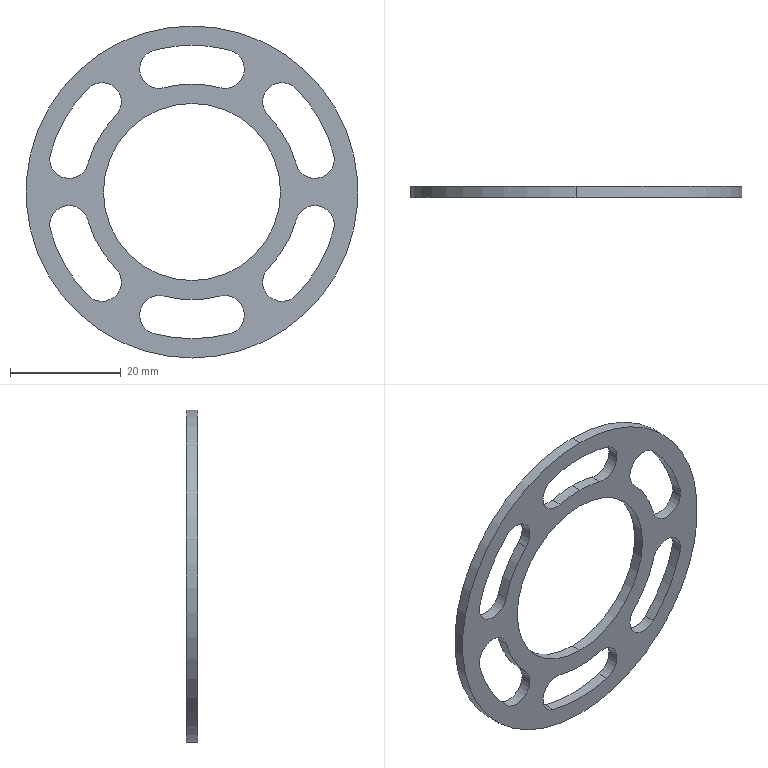Part | SolidWorks | features Extrusion 1, ICE 1 | 1 solid | 38 faces | box 60 x 2 x 60 mm | volume 2573 mm3 | cylinder 36 | plane 2 | commonest cylinder face diameters 7 x18 39 x7 53 x7 32 x2 60 x2
STEP:
#1=CARTESIAN_POINT('',(22.216,0.,-2.453));
#2=VERTEX_POINT('',#1);
#3=CARTESIAN_POINT('',(25.597,0.,-6.859));
#4=VERTEX_POINT('',#3);
#5=CARTESIAN_POINT('',(22.216,0.,-5.953));
#6=DIRECTION('',(0.,1.,0.));
#7=DIRECTION('',(0.,0.,1.));
#8=AXIS2_PLACEMENT_3D('',#5,#6,#7);
#9=CIRCLE('',#8,3.5);
#10=EDGE_CURVE('',#2,#4,#9,.T.);
#11=ORIENTED_EDGE('',*,*,#10,.F.);
#12=CARTESIAN_POINT('',(22.216,2.,-2.453));
#13=VERTEX_POINT('',#12);
#14=CARTESIAN_POINT('',(22.216,0.,-2.453));
#15=DIRECTION('',(0.,1.,0.));
#16=VECTOR('',#15,1000.);
#17=LINE('',#14,#16);
#18=EDGE_CURVE('',#2,#13,#17,.T.);
#19=ORIENTED_EDGE('',*,*,#18,.T.);
#20=CARTESIAN_POINT('',(25.597,2.,-6.859));
#21=VERTEX_POINT('',#20);
#22=CARTESIAN_POINT('',(22.216,2.,-5.953));
#23=DIRECTION('',(0.,1.,0.));
#24=DIRECTION('',(0.,0.,1.));
#25=AXIS2_PLACEMENT_3D('',#22,#23,#24);
#26=CIRCLE('',#25,3.5);
#27=EDGE_CURVE('',#13,#21,#26,.T.);
#28=ORIENTED_EDGE('',*,*,#27,.T.);
#29=CARTESIAN_POINT('',(25.597,0.,-6.859));
#30=DIRECTION('',(0.,1.,0.));
#31=VECTOR('',#30,1000.);
#32=LINE('',#29,#31);
#33=EDGE_CURVE('',#4,#21,#32,.T.);
#34=ORIENTED_EDGE('',*,*,#33,.F.);
#35=EDGE_LOOP('',(#11,#19,#28,#34));
#36=FACE_OUTER_BOUND('',#35,.T.);
#37=CARTESIAN_POINT('',(22.216,0.,-5.953));
#38=DIRECTION('',(0.,1.,0.));
#39=DIRECTION('',(0.,0.,1.));
#40=AXIS2_PLACEMENT_3D('',#37,#38,#39);
#41=CYLINDRICAL_SURFACE('',#40,3.5);
#42=ADVANCED_FACE('',(#36),#41,.F.);
#43=CARTESIAN_POINT('',(16.263,0.,19.763));
#44=VERTEX_POINT('',#43);
#45=CARTESIAN_POINT('',(18.738,0.,18.738));
#46=VERTEX_POINT('',#45);
#47=CARTESIAN_POINT('',(16.263,0.,16.263));
#48=DIRECTION('',(0.,1.,0.));
#49=DIRECTION('',(0.,0.,1.));
#50=AXIS2_PLACEMENT_3D('',#47,#48,#49);
#51=CIRCLE('',#50,3.5);
#52=EDGE_CURVE('',#44,#46,#51,.T.);
#53=ORIENTED_EDGE('',*,*,#52,.F.);
#54=CARTESIAN_POINT('',(16.263,2.,19.763));
#55=VERTEX_POINT('',#54);
#56=CARTESIAN_POINT('',(16.263,0.,19.763));
#57=DIRECTION('',(0.,1.,0.));
#58=VECTOR('',#57,1000.);
#59=LINE('',#56,#58);
#60=EDGE_CURVE('',#44,#55,#59,.T.);
#61=ORIENTED_EDGE('',*,*,#60,.T.);
#62=CARTESIAN_POINT('',(18.738,2.,18.738));
#63=VERTEX_POINT('',#62);
#64=CARTESIAN_POINT('',(16.263,2.,16.263));
#65=DIRECTION('',(0.,1.,0.));
#66=DIRECTION('',(0.,0.,1.));
#67=AXIS2_PLACEMENT_3D('',#64,#65,#66);
#68=CIRCLE('',#67,3.5);
#69=EDGE_CURVE('',#55,#63,#68,.T.);
#70=ORIENTED_EDGE('',*,*,#69,.T.);
#71=CARTESIAN_POINT('',(18.738,0.,18.738));
#72=DIRECTION('',(0.,1.,0.));
#73=VECTOR('',#72,1000.);
#74=LINE('',#71,#73);
#75=EDGE_CURVE('',#46,#63,#74,.T.);
#76=ORIENTED_EDGE('',*,*,#75,.F.);
#77=EDGE_LOOP('',(#53,#61,#70,#76));
#78=FACE_OUTER_BOUND('',#77,.T.);
#79=CARTESIAN_POINT('',(16.263,0.,16.263));
#80=DIRECTION('',(0.,1.,0.));
#81=DIRECTION('',(0.,0.,1.));
#82=AXIS2_PLACEMENT_3D('',#79,#80,#81);
#83=CYLINDRICAL_SURFACE('',#82,3.5);
#84=ADVANCED_FACE('',(#78),#83,.F.);
#85=CARTESIAN_POINT('',(0.,0.,26.5));
#86=VERTEX_POINT('',#85);
#87=CARTESIAN_POINT('',(6.859,0.,25.597));
#88=VERTEX_POINT('',#87);
#89=CARTESIAN_POINT('',(0.,0.,0.));
#90=DIRECTION('',(0.,1.,0.));
#91=DIRECTION('',(0.,0.,1.));
#92=AXIS2_PLACEMENT_3D('',#89,#90,#91);
#93=CIRCLE('',#92,26.5);
#94=EDGE_CURVE('',#86,#88,#93,.T.);
#95=ORIENTED_EDGE('',*,*,#94,.F.);
#96=CARTESIAN_POINT('',(0.,2.,26.5));
#97=VERTEX_POINT('',#96);
#98=CARTESIAN_POINT('',(0.,0.,26.5));
#99=DIRECTION('',(0.,1.,0.));
#100=VECTOR('',#99,1000.);
#101=LINE('',#98,#100);
#102=EDGE_CURVE('',#86,#97,#101,.T.);
#103=ORIENTED_EDGE('',*,*,#102,.T.);
#104=CARTESIAN_POINT('',(6.859,2.,25.597));
#105=VERTEX_POINT('',#104);
#106=CARTESIAN_POINT('',(0.,2.,0.));
#107=DIRECTION('',(0.,1.,0.));
#108=DIRECTION('',(0.,0.,1.));
#109=AXIS2_PLACEMENT_3D('',#106,#107,#108);
#110=CIRCLE('',#109,26.5);
#111=EDGE_CURVE('',#97,#105,#110,.T.);
#112=ORIENTED_EDGE('',*,*,#111,.T.);
#113=CARTESIAN_POINT('',(6.859,0.,25.597));
#114=DIRECTION('',(0.,1.,0.));
#115=VECTOR('',#114,1000.);
#116=LINE('',#113,#115);
#117=EDGE_CURVE('',#88,#105,#116,.T.);
#118=ORIENTED_EDGE('',*,*,#117,.F.);
#119=EDGE_LOOP('',(#95,#103,#112,#118));
#120=FACE_OUTER_BOUND('',#119,.T.);
#121=CARTESIAN_POINT('',(0.,0.,0.));
#122=DIRECTION('',(0.,1.,0.));
#123=DIRECTION('',(0.,0.,1.));
#124=AXIS2_PLACEMENT_3D('',#121,#122,#123);
#125=CYLINDRICAL_SURFACE('',#124,26.5);
#126=ADVANCED_FACE('',(#120),#125,.F.);
#127=CARTESIAN_POINT('',(0.,0.,19.5));
#128=VERTEX_POINT('',#127);
#129=CARTESIAN_POINT('',(-5.047,0.,18.836));
#130=VERTEX_POINT('',#129);
#131=CARTESIAN_POINT('',(0.,0.,0.));
#132=DIRECTION('',(0.,-1.,0.));
#133=DIRECTION('',(0.,0.,1.));
#134=AXIS2_PLACEMENT_3D('',#131,#132,#133);
#135=CIRCLE('',#134,19.5);
#136=EDGE_CURVE('',#128,#130,#135,.T.);
#137=ORIENTED_EDGE('',*,*,#136,.F.);
#138=CARTESIAN_POINT('',(0.,2.,19.5));
#139=VERTEX_POINT('',#138);
#140=CARTESIAN_POINT('',(0.,0.,19.5));
#141=DIRECTION('',(0.,1.,0.));
#142=VECTOR('',#141,1000.);
#143=LINE('',#140,#142);
#144=EDGE_CURVE('',#128,#139,#143,.T.);
#145=ORIENTED_EDGE('',*,*,#144,.T.);
#146=CARTESIAN_POINT('',(-5.047,2.,18.836));
#147=VERTEX_POINT('',#146);
#148=CARTESIAN_POINT('',(0.,2.,0.));
#149=DIRECTION('',(0.,-1.,0.));
#150=DIRECTION('',(0.,0.,1.));
#151=AXIS2_PLACEMENT_3D('',#148,#149,#150);
#152=CIRCLE('',#151,19.5);
#153=EDGE_CURVE('',#139,#147,#152,.T.);
#154=ORIENTED_EDGE('',*,*,#153,.T.);
#155=CARTESIAN_POINT('',(-5.047,0.,18.836));
#156=DIRECTION('',(0.,1.,0.));
#157=VECTOR('',#156,1000.);
#158=LINE('',#155,#157);
#159=EDGE_CURVE('',#130,#147,#158,.T.);
#160=ORIENTED_EDGE('',*,*,#159,.F.);
#161=EDGE_LOOP('',(#137,#145,#154,#160));
#162=FACE_OUTER_BOUND('',#161,.T.);
#163=CARTESIAN_POINT('',(0.,0.,0.));
#164=DIRECTION('',(0.,1.,0.));
#165=DIRECTION('',(0.,0.,1.));
#166=AXIS2_PLACEMENT_3D('',#163,#164,#165);
#167=CYLINDRICAL_SURFACE('',#166,19.5);
#168=ADVANCED_FACE('',(#162),#167,.T.);
#169=CARTESIAN_POINT('',(-16.263,0.,19.763));
#170=VERTEX_POINT('',#169);
#171=CARTESIAN_POINT('',(-13.789,0.,13.789));
#172=VERTEX_POINT('',#171);
#173=CARTESIAN_POINT('',(-16.263,0.,16.263));
#174=DIRECTION('',(0.,1.,0.));
#175=DIRECTION('',(0.,0.,1.));
#176=AXIS2_PLACEMENT_3D('',#173,#174,#175);
#177=CIRCLE('',#176,3.5);
#178=EDGE_CURVE('',#170,#172,#177,.T.);
#179=ORIENTED_EDGE('',*,*,#178,.F.);
#180=CARTESIAN_POINT('',(-16.263,2.,19.763));
#181=VERTEX_POINT('',#180);
#182=CARTESIAN_POINT('',(-16.263,0.,19.763));
#183=DIRECTION('',(0.,1.,0.));
#184=VECTOR('',#183,1000.);
#185=LINE('',#182,#184);
#186=EDGE_CURVE('',#170,#181,#185,.T.);
#187=ORIENTED_EDGE('',*,*,#186,.T.);
#188=CARTESIAN_POINT('',(-13.789,2.,13.789));
#189=VERTEX_POINT('',#188);
#190=CARTESIAN_POINT('',(-16.263,2.,16.263));
#191=DIRECTION('',(0.,1.,0.));
#192=DIRECTION('',(0.,0.,1.));
#193=AXIS2_PLACEMENT_3D('',#190,#191,#192);
#194=CIRCLE('',#193,3.5);
#195=EDGE_CURVE('',#181,#189,#194,.T.);
#196=ORIENTED_EDGE('',*,*,#195,.T.);
#197=CARTESIAN_POINT('',(-13.789,0.,13.789));
#198=DIRECTION('',(0.,1.,0.));
#199=VECTOR('',#198,1000.);
#200=LINE('',#197,#199);
#201=EDGE_CURVE('',#172,#189,#200,.T.);
#202=ORIENTED_EDGE('',*,*,#201,.F.);
#203=EDGE_LOOP('',(#179,#187,#196,#202));
#204=FACE_OUTER_BOUND('',#203,.T.);
#205=CARTESIAN_POINT('',(-16.263,0.,16.263));
#206=DIRECTION('',(0.,1.,0.));
#207=DIRECTION('',(0.,0.,1.));
#208=AXIS2_PLACEMENT_3D('',#205,#206,#207);
#209=CYLINDRICAL_SURFACE('',#208,3.5);
#210=ADVANCED_FACE('',(#204),#209,.F.);
#211=CARTESIAN_POINT('',(-22.216,0.,-2.453));
#212=VERTEX_POINT('',#211);
#213=CARTESIAN_POINT('',(-18.836,0.,-5.047));
#214=VERTEX_POINT('',#213);
#215=CARTESIAN_POINT('',(-22.216,0.,-5.953));
#216=DIRECTION('',(0.,1.,0.));
#217=DIRECTION('',(0.,0.,1.));
#218=AXIS2_PLACEMENT_3D('',#215,#216,#217);
#219=CIRCLE('',#218,3.5);
#220=EDGE_CURVE('',#212,#214,#219,.T.);
#221=ORIENTED_EDGE('',*,*,#220,.F.);
#222=CARTESIAN_POINT('',(-22.216,2.,-2.453));
#223=VERTEX_POINT('',#222);
#224=CARTESIAN_POINT('',(-22.216,0.,-2.453));
#225=DIRECTION('',(0.,1.,0.));
#226=VECTOR('',#225,1000.);
#227=LINE('',#224,#226);
#228=EDGE_CURVE('',#212,#223,#227,.T.);
#229=ORIENTED_EDGE('',*,*,#228,.T.);
#230=CARTESIAN_POINT('',(-18.836,2.,-5.047));
#231=VERTEX_POINT('',#230);
#232=CARTESIAN_POINT('',(-22.216,2.,-5.953));
#233=DIRECTION('',(0.,1.,0.));
#234=DIRECTION('',(0.,0.,1.));
#235=AXIS2_PLACEMENT_3D('',#232,#233,#234);
#236=CIRCLE('',#235,3.5);
#237=EDGE_CURVE('',#223,#231,#236,.T.);
#238=ORIENTED_EDGE('',*,*,#237,.T.);
#239=CARTESIAN_POINT('',(-18.836,0.,-5.047));
#240=DIRECTION('',(0.,1.,0.));
#241=VECTOR('',#240,1000.);
#242=LINE('',#239,#241);
#243=EDGE_CURVE('',#214,#231,#242,.T.);
#244=ORIENTED_EDGE('',*,*,#243,.F.);
#245=EDGE_LOOP('',(#221,#229,#238,#244));
#246=FACE_OUTER_BOUND('',#245,.T.);
#247=CARTESIAN_POINT('',(-22.216,0.,-5.953));
#248=DIRECTION('',(0.,1.,0.));
#249=DIRECTION('',(0.,0.,1.));
#250=AXIS2_PLACEMENT_3D('',#247,#248,#249);
#251=CYLINDRICAL_SURFACE('',#250,3.5);
#252=ADVANCED_FACE('',(#246),#251,.F.);
#253=CARTESIAN_POINT('',(-5.953,0.,-18.716));
#254=VERTEX_POINT('',#253);
#255=CARTESIAN_POINT('',(-5.047,0.,-18.836));
#256=VERTEX_POINT('',#255);
#257=CARTESIAN_POINT('',(-5.953,0.,-22.216));
#258=DIRECTION('',(0.,1.,0.));
#259=DIRECTION('',(0.,0.,1.));
#260=AXIS2_PLACEMENT_3D('',#257,#258,#259);
#261=CIRCLE('',#260,3.5);
#262=EDGE_CURVE('',#254,#256,#261,.T.);
#263=ORIENTED_EDGE('',*,*,#262,.F.);
#264=CARTESIAN_POINT('',(-5.953,2.,-18.716));
#265=VERTEX_POINT('',#264);
#266=CARTESIAN_POINT('',(-5.953,0.,-18.716));
#267=DIRECTION('',(0.,1.,0.));
#268=VECTOR('',#267,1000.);
#269=LINE('',#266,#268);
#270=EDGE_CURVE('',#254,#265,#269,.T.);
#271=ORIENTED_EDGE('',*,*,#270,.T.);
#272=CARTESIAN_POINT('',(-5.047,2.,-18.836));
#273=VERTEX_POINT('',#272);
#274=CARTESIAN_POINT('',(-5.953,2.,-22.216));
#275=DIRECTION('',(0.,1.,0.));
#276=DIRECTION('',(0.,0.,1.));
#277=AXIS2_PLACEMENT_3D('',#274,#275,#276);
#278=CIRCLE('',#277,3.5);
#279=EDGE_CURVE('',#265,#273,#278,.T.);
#280=ORIENTED_EDGE('',*,*,#279,.T.);
#281=CARTESIAN_POINT('',(-5.047,0.,-18.836));
#282=DIRECTION('',(0.,1.,0.));
#283=VECTOR('',#282,1000.);
#284=LINE('',#281,#283);
#285=EDGE_CURVE('',#256,#273,#284,.T.);
#286=ORIENTED_EDGE('',*,*,#285,.F.);
#287=EDGE_LOOP('',(#263,#271,#280,#286));
#288=FACE_OUTER_BOUND('',#287,.T.);
#289=CARTESIAN_POINT('',(-5.953,0.,-22.216));
#290=DIRECTION('',(0.,1.,0.));
#291=DIRECTION('',(0.,0.,1.));
#292=AXIS2_PLACEMENT_3D('',#289,#290,#291);
#293=CYLINDRICAL_SURFACE('',#292,3.5);
#294=ADVANCED_FACE('',(#288),#293,.F.);
#295=CARTESIAN_POINT('',(5.953,0.,-18.716));
#296=VERTEX_POINT('',#295);
#297=CARTESIAN_POINT('',(6.859,0.,-25.597));
#298=VERTEX_POINT('',#297);
#299=CARTESIAN_POINT('',(5.953,0.,-22.216));
#300=DIRECTION('',(0.,1.,0.));
#301=DIRECTION('',(0.,0.,1.));
#302=AXIS2_PLACEMENT_3D('',#299,#300,#301);
#303=CIRCLE('',#302,3.5);
#304=EDGE_CURVE('',#296,#298,#303,.T.);
#305=ORIENTED_EDGE('',*,*,#304,.F.);
#306=CARTESIAN_POINT('',(5.953,2.,-18.716));
#307=VERTEX_POINT('',#306);
#308=CARTESIAN_POINT('',(5.953,0.,-18.716));
#309=DIRECTION('',(0.,1.,0.));
#310=VECTOR('',#309,1000.);
#311=LINE('',#308,#310);
#312=EDGE_CURVE('',#296,#307,#311,.T.);
#313=ORIENTED_EDGE('',*,*,#312,.T.);
#314=CARTESIAN_POINT('',(6.859,2.,-25.597));
#315=VERTEX_POINT('',#314);
#316=CARTESIAN_POINT('',(5.953,2.,-22.216));
#317=DIRECTION('',(0.,1.,0.));
#318=DIRECTION('',(0.,0.,1.));
#319=AXIS2_PLACEMENT_3D('',#316,#317,#318);
#320=CIRCLE('',#319,3.5);
#321=EDGE_CURVE('',#307,#315,#320,.T.);
#322=ORIENTED_EDGE('',*,*,#321,.T.);
#323=CARTESIAN_POINT('',(6.859,0.,-25.597));
#324=DIRECTION('',(0.,1.,0.));
#325=VECTOR('',#324,1000.);
#326=LINE('',#323,#325);
#327=EDGE_CURVE('',#298,#315,#326,.T.);
#328=ORIENTED_EDGE('',*,*,#327,.F.);
#329=EDGE_LOOP('',(#305,#313,#322,#328));
#330=FACE_OUTER_BOUND('',#329,.T.);
#331=CARTESIAN_POINT('',(5.953,0.,-22.216));
#332=DIRECTION('',(0.,1.,0.));
#333=DIRECTION('',(0.,0.,1.));
#334=AXIS2_PLACEMENT_3D('',#331,#332,#333);
#335=CYLINDRICAL_SURFACE('',#334,3.5);
#336=ADVANCED_FACE('',(#330),#335,.F.);
#337=CARTESIAN_POINT('',(0.,2.,-16.));
#338=VERTEX_POINT('',#337);
#339=CARTESIAN_POINT('',(0.,2.,16.));
#340=VERTEX_POINT('',#339);
#341=CARTESIAN_POINT('',(0.,2.,0.));
#342=DIRECTION('',(0.,1.,0.));
#343=DIRECTION('',(0.,0.,1.));
#344=AXIS2_PLACEMENT_3D('',#341,#342,#343);
#345=CIRCLE('',#344,16.);
#346=EDGE_CURVE('',#338,#340,#345,.T.);
#347=ORIENTED_EDGE('',*,*,#346,.T.);
#348=CARTESIAN_POINT('',(0.,0.,16.));
#349=VERTEX_POINT('',#348);
#350=CARTESIAN_POINT('',(0.,2.,16.));
#351=DIRECTION('',(0.,-1.,0.));
#352=VECTOR('',#351,1000.);
#353=LINE('',#350,#352);
#354=EDGE_CURVE('',#340,#349,#353,.T.);
#355=ORIENTED_EDGE('',*,*,#354,.T.);
#356=CARTESIAN_POINT('',(0.,0.,-16.));
#357=VERTEX_POINT('',#356);
#358=CARTESIAN_POINT('',(0.,0.,0.));
#359=DIRECTION('',(0.,1.,0.));
#360=DIRECTION('',(0.,0.,1.));
#361=AXIS2_PLACEMENT_3D('',#358,#359,#360);
#362=CIRCLE('',#361,16.);
#363=EDGE_CURVE('',#357,#349,#362,.T.);
#364=ORIENTED_EDGE('',*,*,#363,.F.);
#365=CARTESIAN_POINT('',(0.,2.,-16.));
#366=DIRECTION('',(0.,-1.,0.));
#367=VECTOR('',#366,1000.);
#368=LINE('',#365,#367);
#369=EDGE_CURVE('',#338,#357,#368,.T.);
#370=ORIENTED_EDGE('',*,*,#369,.F.);
#371=EDGE_LOOP('',(#347,#355,#364,#370));
#372=FACE_OUTER_BOUND('',#371,.T.);
#373=CARTESIAN_POINT('',(0.,2.,0.));
#374=DIRECTION('',(0.,-1.,0.));
#375=DIRECTION('',(0.,0.,-1.));
#376=AXIS2_PLACEMENT_3D('',#373,#374,#375);
#377=CYLINDRICAL_SURFACE('',#376,16.);
#378=ADVANCED_FACE('',(#372),#377,.F.);
#379=CARTESIAN_POINT('',(0.,2.,30.));
#380=VERTEX_POINT('',#379);
#381=CARTESIAN_POINT('',(0.,2.,-30.));
#382=VERTEX_POINT('',#381);
#383=CARTESIAN_POINT('',(0.,2.,0.));
#384=DIRECTION('',(0.,1.,0.));
#385=DIRECTION('',(0.,0.,1.));
#386=AXIS2_PLACEMENT_3D('',#383,#384,#385);
#387=CIRCLE('',#386,30.);
#388=EDGE_CURVE('',#380,#382,#387,.T.);
#389=ORIENTED_EDGE('',*,*,#388,.F.);
#390=CARTESIAN_POINT('',(0.,0.,30.));
#391=VERTEX_POINT('',#390);
#392=CARTESIAN_POINT('',(0.,2.,30.));
#393=DIRECTION('',(0.,-1.,0.));
#394=VECTOR('',#393,1000.);
#395=LINE('',#392,#394);
#396=EDGE_CURVE('',#380,#391,#395,.T.);
#397=ORIENTED_EDGE('',*,*,#396,.T.);
#398=CARTESIAN_POINT('',(0.,0.,-30.));
#399=VERTEX_POINT('',#398);
#400=CARTESIAN_POINT('',(0.,0.,0.));
#401=DIRECTION('',(0.,1.,0.));
#402=DIRECTION('',(0.,0.,1.));
#403=AXIS2_PLACEMENT_3D('',#400,#401,#402);
#404=CIRCLE('',#403,30.);
#405=EDGE_CURVE('',#391,#399,#404,.T.);
#406=ORIENTED_EDGE('',*,*,#405,.T.);
#407=CARTESIAN_POINT('',(0.,2.,-30.));
#408=DIRECTION('',(0.,-1.,0.));
#409=VECTOR('',#408,1000.);
#410=LINE('',#407,#409);
#411=EDGE_CURVE('',#382,#399,#410,.T.);
#412=ORIENTED_EDGE('',*,*,#411,.F.);
#413=EDGE_LOOP('',(#389,#397,#406,#412));
#414=FACE_OUTER_BOUND('',#413,.T.);
#415=CARTESIAN_POINT('',(0.,2.,0.));
#416=DIRECTION('',(0.,-1.,0.));
#417=DIRECTION('',(0.,0.,-1.));
#418=AXIS2_PLACEMENT_3D('',#415,#416,#417);
#419=CYLINDRICAL_SURFACE('',#418,30.);
#420=ADVANCED_FACE('',(#414),#419,.T.);
#421=CARTESIAN_POINT('',(18.836,2.,-5.047));
#422=VERTEX_POINT('',#421);
#423=CARTESIAN_POINT('',(22.216,2.,-5.953));
#424=DIRECTION('',(0.,1.,0.));
#425=DIRECTION('',(0.,0.,1.));
#426=AXIS2_PLACEMENT_3D('',#423,#424,#425);
#427=CIRCLE('',#426,3.5);
#428=EDGE_CURVE('',#422,#13,#427,.T.);
#429=ORIENTED_EDGE('',*,*,#428,.F.);
#430=CARTESIAN_POINT('',(13.789,2.,-13.789));
#431=VERTEX_POINT('',#430);
#432=CARTESIAN_POINT('',(0.,2.,0.));
#433=DIRECTION('',(0.,-1.,0.));
#434=DIRECTION('',(0.,0.,1.));
#435=AXIS2_PLACEMENT_3D('',#432,#433,#434);
#436=CIRCLE('',#435,19.5);
#437=EDGE_CURVE('',#431,#422,#436,.T.);
#438=ORIENTED_EDGE('',*,*,#437,.F.);
#439=CARTESIAN_POINT('',(18.738,2.,-18.738));
#440=VERTEX_POINT('',#439);
#441=CARTESIAN_POINT('',(16.263,2.,-16.263));
#442=DIRECTION('',(0.,1.,0.));
#443=DIRECTION('',(0.,0.,1.));
#444=AXIS2_PLACEMENT_3D('',#441,#442,#443);
#445=CIRCLE('',#444,3.5);
#446=EDGE_CURVE('',#440,#431,#445,.T.);
#447=ORIENTED_EDGE('',*,*,#446,.F.);
#448=CARTESIAN_POINT('',(0.,2.,0.));
#449=DIRECTION('',(0.,1.,0.));
#450=DIRECTION('',(0.,0.,1.));
#451=AXIS2_PLACEMENT_3D('',#448,#449,#450);
#452=CIRCLE('',#451,26.5);
#453=EDGE_CURVE('',#21,#440,#452,.T.);
#454=ORIENTED_EDGE('',*,*,#453,.F.);
#455=ORIENTED_EDGE('',*,*,#27,.F.);
#456=EDGE_LOOP('',(#429,#438,#447,#454,#455));
#457=FACE_BOUND('',#456,.T.);
#458=CARTESIAN_POINT('',(13.789,2.,13.789));
#459=VERTEX_POINT('',#458);
#460=CARTESIAN_POINT('',(16.263,2.,16.263));
#461=DIRECTION('',(0.,1.,0.));
#462=DIRECTION('',(0.,0.,1.));
#463=AXIS2_PLACEMENT_3D('',#460,#461,#462);
#464=CIRCLE('',#463,3.5);
#465=EDGE_CURVE('',#459,#55,#464,.T.);
#466=ORIENTED_EDGE('',*,*,#465,.F.);
#467=CARTESIAN_POINT('',(18.836,2.,5.047));
#468=VERTEX_POINT('',#467);
#469=CARTESIAN_POINT('',(0.,2.,0.));
#470=DIRECTION('',(0.,-1.,0.));
#471=DIRECTION('',(0.,0.,1.));
#472=AXIS2_PLACEMENT_3D('',#469,#470,#471);
#473=CIRCLE('',#472,19.5);
#474=EDGE_CURVE('',#468,#459,#473,.T.);
#475=ORIENTED_EDGE('',*,*,#474,.F.);
#476=CARTESIAN_POINT('',(25.597,2.,6.859));
#477=VERTEX_POINT('',#476);
#478=CARTESIAN_POINT('',(22.216,2.,5.953));
#479=DIRECTION('',(0.,1.,0.));
#480=DIRECTION('',(0.,0.,1.));
#481=AXIS2_PLACEMENT_3D('',#478,#479,#480);
#482=CIRCLE('',#481,3.5);
#483=EDGE_CURVE('',#477,#468,#482,.T.);
#484=ORIENTED_EDGE('',*,*,#483,.F.);
#485=CARTESIAN_POINT('',(0.,2.,0.));
#486=DIRECTION('',(0.,1.,0.));
#487=DIRECTION('',(0.,0.,1.));
#488=AXIS2_PLACEMENT_3D('',#485,#486,#487);
#489=CIRCLE('',#488,26.5);
#490=EDGE_CURVE('',#63,#477,#489,.T.);
#491=ORIENTED_EDGE('',*,*,#490,.F.);
#492=ORIENTED_EDGE('',*,*,#69,.F.);
#493=EDGE_LOOP('',(#466,#475,#484,#491,#492));
#494=FACE_BOUND('',#493,.T.);
#495=CARTESIAN_POINT('',(-6.859,2.,25.597));
#496=VERTEX_POINT('',#495);
#497=CARTESIAN_POINT('',(-5.953,2.,22.216));
#498=DIRECTION('',(0.,1.,0.));
#499=DIRECTION('',(0.,0.,1.));
#500=AXIS2_PLACEMENT_3D('',#497,#498,#499);
#501=CIRCLE('',#500,3.5);
#502=EDGE_CURVE('',#147,#496,#501,.T.);
#503=ORIENTED_EDGE('',*,*,#502,.F.);
#504=ORIENTED_EDGE('',*,*,#153,.F.);
#505=CARTESIAN_POINT('',(5.047,2.,18.836));
#506=VERTEX_POINT('',#505);
#507=CARTESIAN_POINT('',(0.,2.,0.));
#508=DIRECTION('',(0.,-1.,0.));
#509=DIRECTION('',(0.,0.,1.));
#510=AXIS2_PLACEMENT_3D('',#507,#508,#509);
#511=CIRCLE('',#510,19.5);
#512=EDGE_CURVE('',#506,#139,#511,.T.);
#513=ORIENTED_EDGE('',*,*,#512,.F.);
#514=CARTESIAN_POINT('',(5.953,2.,22.216));
#515=DIRECTION('',(0.,1.,0.));
#516=DIRECTION('',(0.,0.,1.));
#517=AXIS2_PLACEMENT_3D('',#514,#515,#516);
#518=CIRCLE('',#517,3.5);
#519=EDGE_CURVE('',#105,#506,#518,.T.);
#520=ORIENTED_EDGE('',*,*,#519,.F.);
#521=ORIENTED_EDGE('',*,*,#111,.F.);
#522=CARTESIAN_POINT('',(0.,2.,0.));
#523=DIRECTION('',(0.,1.,0.));
#524=DIRECTION('',(0.,0.,1.));
#525=AXIS2_PLACEMENT_3D('',#522,#523,#524);
#526=CIRCLE('',#525,26.5);
#527=EDGE_CURVE('',#496,#97,#526,.T.);
#528=ORIENTED_EDGE('',*,*,#527,.F.);
#529=EDGE_LOOP('',(#503,#504,#513,#520,#521,#528));
#530=FACE_BOUND('',#529,.T.);
#531=CARTESIAN_POINT('',(-18.836,2.,5.047));
#532=VERTEX_POINT('',#531);
#533=CARTESIAN_POINT('',(-25.597,2.,6.859));
#534=VERTEX_POINT('',#533);
#535=CARTESIAN_POINT('',(-22.216,2.,5.953));
#536=DIRECTION('',(0.,1.,0.));
#537=DIRECTION('',(0.,0.,1.));
#538=AXIS2_PLACEMENT_3D('',#535,#536,#537);
#539=CIRCLE('',#538,3.5);
#540=EDGE_CURVE('',#532,#534,#539,.T.);
#541=ORIENTED_EDGE('',*,*,#540,.F.);
#542=CARTESIAN_POINT('',(0.,2.,0.));
#543=DIRECTION('',(0.,-1.,0.));
#544=DIRECTION('',(0.,0.,1.));
#545=AXIS2_PLACEMENT_3D('',#542,#543,#544);
#546=CIRCLE('',#545,19.5);
#547=EDGE_CURVE('',#189,#532,#546,.T.);
#548=ORIENTED_EDGE('',*,*,#547,.F.);
#549=ORIENTED_EDGE('',*,*,#195,.F.);
#550=CARTESIAN_POINT('',(-18.738,2.,18.738));
#551=VERTEX_POINT('',#550);
#552=CARTESIAN_POINT('',(-16.263,2.,16.263));
#553=DIRECTION('',(0.,1.,0.));
#554=DIRECTION('',(0.,0.,1.));
#555=AXIS2_PLACEMENT_3D('',#552,#553,#554);
#556=CIRCLE('',#555,3.5);
#557=EDGE_CURVE('',#551,#181,#556,.T.);
#558=ORIENTED_EDGE('',*,*,#557,.F.);
#559=CARTESIAN_POINT('',(0.,2.,0.));
#560=DIRECTION('',(0.,1.,0.));
#561=DIRECTION('',(0.,0.,1.));
#562=AXIS2_PLACEMENT_3D('',#559,#560,#561);
#563=CIRCLE('',#562,26.5);
#564=EDGE_CURVE('',#534,#551,#563,.T.);
#565=ORIENTED_EDGE('',*,*,#564,.F.);
#566=EDGE_LOOP('',(#541,#548,#549,#558,#565));
#567=FACE_BOUND('',#566,.T.);
#568=CARTESIAN_POINT('',(-13.789,2.,-13.789));
#569=VERTEX_POINT('',#568);
#570=CARTESIAN_POINT('',(-18.738,2.,-18.738));
#571=VERTEX_POINT('',#570);
#572=CARTESIAN_POINT('',(-16.263,2.,-16.263));
#573=DIRECTION('',(0.,1.,0.));
#574=DIRECTION('',(0.,0.,1.));
#575=AXIS2_PLACEMENT_3D('',#572,#573,#574);
#576=CIRCLE('',#575,3.5);
#577=EDGE_CURVE('',#569,#571,#576,.T.);
#578=ORIENTED_EDGE('',*,*,#577,.F.);
#579=CARTESIAN_POINT('',(0.,2.,0.));
#580=DIRECTION('',(0.,-1.,0.));
#581=DIRECTION('',(0.,0.,1.));
#582=AXIS2_PLACEMENT_3D('',#579,#580,#581);
#583=CIRCLE('',#582,19.5);
#584=EDGE_CURVE('',#231,#569,#583,.T.);
#585=ORIENTED_EDGE('',*,*,#584,.F.);
#586=ORIENTED_EDGE('',*,*,#237,.F.);
#587=CARTESIAN_POINT('',(-25.597,2.,-6.859));
#588=VERTEX_POINT('',#587);
#589=CARTESIAN_POINT('',(-22.216,2.,-5.953));
#590=DIRECTION('',(0.,1.,0.));
#591=DIRECTION('',(0.,0.,1.));
#592=AXIS2_PLACEMENT_3D('',#589,#590,#591);
#593=CIRCLE('',#592,3.5);
#594=EDGE_CURVE('',#588,#223,#593,.T.);
#595=ORIENTED_EDGE('',*,*,#594,.F.);
#596=CARTESIAN_POINT('',(0.,2.,0.));
#597=DIRECTION('',(0.,1.,0.));
#598=DIRECTION('',(0.,0.,1.));
#599=AXIS2_PLACEMENT_3D('',#596,#597,#598);
#600=CIRCLE('',#599,26.5);
#601=EDGE_CURVE('',#571,#588,#600,.T.);
#602=ORIENTED_EDGE('',*,*,#601,.F.);
#603=EDGE_LOOP('',(#578,#585,#586,#595,#602));
#604=FACE_BOUND('',#603,.T.);
#605=CARTESIAN_POINT('',(5.047,2.,-18.836));
#606=VERTEX_POINT('',#605);
#607=CARTESIAN_POINT('',(5.953,2.,-22.216));
#608=DIRECTION('',(0.,1.,0.));
#609=DIRECTION('',(0.,0.,1.));
#610=AXIS2_PLACEMENT_3D('',#607,#608,#609);
#611=CIRCLE('',#610,3.5);
#612=EDGE_CURVE('',#606,#307,#611,.T.);
#613=ORIENTED_EDGE('',*,*,#612,.F.);
#614=CARTESIAN_POINT('',(0.,2.,0.));
#615=DIRECTION('',(0.,-1.,0.));
#616=DIRECTION('',(0.,0.,1.));
#617=AXIS2_PLACEMENT_3D('',#614,#615,#616);
#618=CIRCLE('',#617,19.5);
#619=EDGE_CURVE('',#273,#606,#618,.T.);
#620=ORIENTED_EDGE('',*,*,#619,.F.);
#621=ORIENTED_EDGE('',*,*,#279,.F.);
#622=CARTESIAN_POINT('',(-6.859,2.,-25.597));
#623=VERTEX_POINT('',#622);
#624=CARTESIAN_POINT('',(-5.953,2.,-22.216));
#625=DIRECTION('',(0.,1.,0.));
#626=DIRECTION('',(0.,0.,1.));
#627=AXIS2_PLACEMENT_3D('',#624,#625,#626);
#628=CIRCLE('',#627,3.5);
#629=EDGE_CURVE('',#623,#265,#628,.T.);
#630=ORIENTED_EDGE('',*,*,#629,.F.);
#631=CARTESIAN_POINT('',(0.,2.,0.));
#632=DIRECTION('',(0.,1.,0.));
#633=DIRECTION('',(0.,0.,1.));
#634=AXIS2_PLACEMENT_3D('',#631,#632,#633);
#635=CIRCLE('',#634,26.5);
#636=EDGE_CURVE('',#315,#623,#635,.T.);
#637=ORIENTED_EDGE('',*,*,#636,.F.);
#638=ORIENTED_EDGE('',*,*,#321,.F.);
#639=EDGE_LOOP('',(#613,#620,#621,#630,#637,#638));
#640=FACE_BOUND('',#639,.T.);
#641=CARTESIAN_POINT('',(0.,2.,0.));
#642=DIRECTION('',(0.,1.,0.));
#643=DIRECTION('',(0.,0.,1.));
#644=AXIS2_PLACEMENT_3D('',#641,#642,#643);
#645=CIRCLE('',#644,30.);
#646=EDGE_CURVE('',#382,#380,#645,.T.);
#647=ORIENTED_EDGE('',*,*,#646,.T.);
#648=ORIENTED_EDGE('',*,*,#388,.T.);
#649=EDGE_LOOP('',(#647,#648));
#650=FACE_OUTER_BOUND('',#649,.T.);
#651=ORIENTED_EDGE('',*,*,#346,.F.);
#652=CARTESIAN_POINT('',(0.,2.,0.));
#653=DIRECTION('',(0.,1.,0.));
#654=DIRECTION('',(0.,0.,1.));
#655=AXIS2_PLACEMENT_3D('',#652,#653,#654);
#656=CIRCLE('',#655,16.);
#657=EDGE_CURVE('',#340,#338,#656,.T.);
#658=ORIENTED_EDGE('',*,*,#657,.F.);
#659=EDGE_LOOP('',(#651,#658));
#660=FACE_BOUND('',#659,.T.);
#661=CARTESIAN_POINT('',(0.,2.,0.));
#662=DIRECTION('',(0.,1.,0.));
#663=DIRECTION('',(0.,0.,1.));
#664=AXIS2_PLACEMENT_3D('',#661,#662,#663);
#665=PLANE('',#664);
#666=ADVANCED_FACE('',(#457,#494,#530,#567,#604,#640,#650,#660),#665,.T.);
#667=CARTESIAN_POINT('',(13.789,0.,-13.789));
#668=VERTEX_POINT('',#667);
#669=CARTESIAN_POINT('',(18.836,0.,-5.047));
#670=VERTEX_POINT('',#669);
#671=CARTESIAN_POINT('',(0.,0.,0.));
#672=DIRECTION('',(0.,-1.,0.));
#673=DIRECTION('',(0.,0.,1.));
#674=AXIS2_PLACEMENT_3D('',#671,#672,#673);
#675=CIRCLE('',#674,19.5);
#676=EDGE_CURVE('',#668,#670,#675,.T.);
#677=ORIENTED_EDGE('',*,*,#676,.T.);
#678=CARTESIAN_POINT('',(22.216,0.,-5.953));
#679=DIRECTION('',(0.,1.,0.));
#680=DIRECTION('',(0.,0.,1.));
#681=AXIS2_PLACEMENT_3D('',#678,#679,#680);
#682=CIRCLE('',#681,3.5);
#683=EDGE_CURVE('',#670,#2,#682,.T.);
#684=ORIENTED_EDGE('',*,*,#683,.T.);
#685=ORIENTED_EDGE('',*,*,#10,.T.);
#686=CARTESIAN_POINT('',(18.738,0.,-18.738));
#687=VERTEX_POINT('',#686);
#688=CARTESIAN_POINT('',(0.,0.,0.));
#689=DIRECTION('',(0.,1.,0.));
#690=DIRECTION('',(0.,0.,1.));
#691=AXIS2_PLACEMENT_3D('',#688,#689,#690);
#692=CIRCLE('',#691,26.5);
#693=EDGE_CURVE('',#4,#687,#692,.T.);
#694=ORIENTED_EDGE('',*,*,#693,.T.);
#695=CARTESIAN_POINT('',(16.263,0.,-16.263));
#696=DIRECTION('',(0.,1.,0.));
#697=DIRECTION('',(0.,0.,1.));
#698=AXIS2_PLACEMENT_3D('',#695,#696,#697);
#699=CIRCLE('',#698,3.5);
#700=EDGE_CURVE('',#687,#668,#699,.T.);
#701=ORIENTED_EDGE('',*,*,#700,.T.);
#702=EDGE_LOOP('',(#677,#684,#685,#694,#701));
#703=FACE_BOUND('',#702,.T.);
#704=CARTESIAN_POINT('',(18.836,0.,5.047));
#705=VERTEX_POINT('',#704);
#706=CARTESIAN_POINT('',(13.789,0.,13.789));
#707=VERTEX_POINT('',#706);
#708=CARTESIAN_POINT('',(0.,0.,0.));
#709=DIRECTION('',(0.,-1.,0.));
#710=DIRECTION('',(0.,0.,1.));
#711=AXIS2_PLACEMENT_3D('',#708,#709,#710);
#712=CIRCLE('',#711,19.5);
#713=EDGE_CURVE('',#705,#707,#712,.T.);
#714=ORIENTED_EDGE('',*,*,#713,.T.);
#715=CARTESIAN_POINT('',(16.263,0.,16.263));
#716=DIRECTION('',(0.,1.,0.));
#717=DIRECTION('',(0.,0.,1.));
#718=AXIS2_PLACEMENT_3D('',#715,#716,#717);
#719=CIRCLE('',#718,3.5);
#720=EDGE_CURVE('',#707,#44,#719,.T.);
#721=ORIENTED_EDGE('',*,*,#720,.T.);
#722=ORIENTED_EDGE('',*,*,#52,.T.);
#723=CARTESIAN_POINT('',(25.597,0.,6.859));
#724=VERTEX_POINT('',#723);
#725=CARTESIAN_POINT('',(0.,0.,0.));
#726=DIRECTION('',(0.,1.,0.));
#727=DIRECTION('',(0.,0.,1.));
#728=AXIS2_PLACEMENT_3D('',#725,#726,#727);
#729=CIRCLE('',#728,26.5);
#730=EDGE_CURVE('',#46,#724,#729,.T.);
#731=ORIENTED_EDGE('',*,*,#730,.T.);
#732=CARTESIAN_POINT('',(22.216,0.,5.953));
#733=DIRECTION('',(0.,1.,0.));
#734=DIRECTION('',(0.,0.,1.));
#735=AXIS2_PLACEMENT_3D('',#732,#733,#734);
#736=CIRCLE('',#735,3.5);
#737=EDGE_CURVE('',#724,#705,#736,.T.);
#738=ORIENTED_EDGE('',*,*,#737,.T.);
#739=EDGE_LOOP('',(#714,#721,#722,#731,#738));
#740=FACE_BOUND('',#739,.T.);
#741=CARTESIAN_POINT('',(5.047,0.,18.836));
#742=VERTEX_POINT('',#741);
#743=CARTESIAN_POINT('',(0.,0.,0.));
#744=DIRECTION('',(0.,-1.,0.));
#745=DIRECTION('',(0.,0.,1.));
#746=AXIS2_PLACEMENT_3D('',#743,#744,#745);
#747=CIRCLE('',#746,19.5);
#748=EDGE_CURVE('',#742,#128,#747,.T.);
#749=ORIENTED_EDGE('',*,*,#748,.T.);
#750=ORIENTED_EDGE('',*,*,#136,.T.);
#751=CARTESIAN_POINT('',(-6.859,0.,25.597));
#752=VERTEX_POINT('',#751);
#753=CARTESIAN_POINT('',(-5.953,0.,22.216));
#754=DIRECTION('',(0.,1.,0.));
#755=DIRECTION('',(0.,0.,1.));
#756=AXIS2_PLACEMENT_3D('',#753,#754,#755);
#757=CIRCLE('',#756,3.5);
#758=EDGE_CURVE('',#130,#752,#757,.T.);
#759=ORIENTED_EDGE('',*,*,#758,.T.);
#760=CARTESIAN_POINT('',(0.,0.,0.));
#761=DIRECTION('',(0.,1.,0.));
#762=DIRECTION('',(0.,0.,1.));
#763=AXIS2_PLACEMENT_3D('',#760,#761,#762);
#764=CIRCLE('',#763,26.5);
#765=EDGE_CURVE('',#752,#86,#764,.T.);
#766=ORIENTED_EDGE('',*,*,#765,.T.);
#767=ORIENTED_EDGE('',*,*,#94,.T.);
#768=CARTESIAN_POINT('',(5.953,0.,22.216));
#769=DIRECTION('',(0.,1.,0.));
#770=DIRECTION('',(0.,0.,1.));
#771=AXIS2_PLACEMENT_3D('',#768,#769,#770);
#772=CIRCLE('',#771,3.5);
#773=EDGE_CURVE('',#88,#742,#772,.T.);
#774=ORIENTED_EDGE('',*,*,#773,.T.);
#775=EDGE_LOOP('',(#749,#750,#759,#766,#767,#774));
#776=FACE_BOUND('',#775,.T.);
#777=CARTESIAN_POINT('',(-18.836,0.,5.047));
#778=VERTEX_POINT('',#777);
#779=CARTESIAN_POINT('',(0.,0.,0.));
#780=DIRECTION('',(0.,-1.,0.));
#781=DIRECTION('',(0.,0.,1.));
#782=AXIS2_PLACEMENT_3D('',#779,#780,#781);
#783=CIRCLE('',#782,19.5);
#784=EDGE_CURVE('',#172,#778,#783,.T.);
#785=ORIENTED_EDGE('',*,*,#784,.T.);
#786=CARTESIAN_POINT('',(-25.597,0.,6.859));
#787=VERTEX_POINT('',#786);
#788=CARTESIAN_POINT('',(-22.216,0.,5.953));
#789=DIRECTION('',(0.,1.,0.));
#790=DIRECTION('',(0.,0.,1.));
#791=AXIS2_PLACEMENT_3D('',#788,#789,#790);
#792=CIRCLE('',#791,3.5);
#793=EDGE_CURVE('',#778,#787,#792,.T.);
#794=ORIENTED_EDGE('',*,*,#793,.T.);
#795=CARTESIAN_POINT('',(-18.738,0.,18.738));
#796=VERTEX_POINT('',#795);
#797=CARTESIAN_POINT('',(0.,0.,0.));
#798=DIRECTION('',(0.,1.,0.));
#799=DIRECTION('',(0.,0.,1.));
#800=AXIS2_PLACEMENT_3D('',#797,#798,#799);
#801=CIRCLE('',#800,26.5);
#802=EDGE_CURVE('',#787,#796,#801,.T.);
#803=ORIENTED_EDGE('',*,*,#802,.T.);
#804=CARTESIAN_POINT('',(-16.263,0.,16.263));
#805=DIRECTION('',(0.,1.,0.));
#806=DIRECTION('',(0.,0.,1.));
#807=AXIS2_PLACEMENT_3D('',#804,#805,#806);
#808=CIRCLE('',#807,3.5);
#809=EDGE_CURVE('',#796,#170,#808,.T.);
#810=ORIENTED_EDGE('',*,*,#809,.T.);
#811=ORIENTED_EDGE('',*,*,#178,.T.);
#812=EDGE_LOOP('',(#785,#794,#803,#810,#811));
#813=FACE_BOUND('',#812,.T.);
#814=CARTESIAN_POINT('',(-13.789,0.,-13.789));
#815=VERTEX_POINT('',#814);
#816=CARTESIAN_POINT('',(0.,0.,0.));
#817=DIRECTION('',(0.,-1.,0.));
#818=DIRECTION('',(0.,0.,1.));
#819=AXIS2_PLACEMENT_3D('',#816,#817,#818);
#820=CIRCLE('',#819,19.5);
#821=EDGE_CURVE('',#214,#815,#820,.T.);
#822=ORIENTED_EDGE('',*,*,#821,.T.);
#823=CARTESIAN_POINT('',(-18.738,0.,-18.738));
#824=VERTEX_POINT('',#823);
#825=CARTESIAN_POINT('',(-16.263,0.,-16.263));
#826=DIRECTION('',(0.,1.,0.));
#827=DIRECTION('',(0.,0.,1.));
#828=AXIS2_PLACEMENT_3D('',#825,#826,#827);
#829=CIRCLE('',#828,3.5);
#830=EDGE_CURVE('',#815,#824,#829,.T.);
#831=ORIENTED_EDGE('',*,*,#830,.T.);
#832=CARTESIAN_POINT('',(-25.597,0.,-6.859));
#833=VERTEX_POINT('',#832);
#834=CARTESIAN_POINT('',(0.,0.,0.));
#835=DIRECTION('',(0.,1.,0.));
#836=DIRECTION('',(0.,0.,1.));
#837=AXIS2_PLACEMENT_3D('',#834,#835,#836);
#838=CIRCLE('',#837,26.5);
#839=EDGE_CURVE('',#824,#833,#838,.T.);
#840=ORIENTED_EDGE('',*,*,#839,.T.);
#841=CARTESIAN_POINT('',(-22.216,0.,-5.953));
#842=DIRECTION('',(0.,1.,0.));
#843=DIRECTION('',(0.,0.,1.));
#844=AXIS2_PLACEMENT_3D('',#841,#842,#843);
#845=CIRCLE('',#844,3.5);
#846=EDGE_CURVE('',#833,#212,#845,.T.);
#847=ORIENTED_EDGE('',*,*,#846,.T.);
#848=ORIENTED_EDGE('',*,*,#220,.T.);
#849=EDGE_LOOP('',(#822,#831,#840,#847,#848));
#850=FACE_BOUND('',#849,.T.);
#851=CARTESIAN_POINT('',(5.047,0.,-18.836));
#852=VERTEX_POINT('',#851);
#853=CARTESIAN_POINT('',(0.,0.,0.));
#854=DIRECTION('',(0.,-1.,0.));
#855=DIRECTION('',(0.,0.,1.));
#856=AXIS2_PLACEMENT_3D('',#853,#854,#855);
#857=CIRCLE('',#856,19.5);
#858=EDGE_CURVE('',#256,#852,#857,.T.);
#859=ORIENTED_EDGE('',*,*,#858,.T.);
#860=CARTESIAN_POINT('',(5.953,0.,-22.216));
#861=DIRECTION('',(0.,1.,0.));
#862=DIRECTION('',(0.,0.,1.));
#863=AXIS2_PLACEMENT_3D('',#860,#861,#862);
#864=CIRCLE('',#863,3.5);
#865=EDGE_CURVE('',#852,#296,#864,.T.);
#866=ORIENTED_EDGE('',*,*,#865,.T.);
#867=ORIENTED_EDGE('',*,*,#304,.T.);
#868=CARTESIAN_POINT('',(-6.859,0.,-25.597));
#869=VERTEX_POINT('',#868);
#870=CARTESIAN_POINT('',(0.,0.,0.));
#871=DIRECTION('',(0.,1.,0.));
#872=DIRECTION('',(0.,0.,1.));
#873=AXIS2_PLACEMENT_3D('',#870,#871,#872);
#874=CIRCLE('',#873,26.5);
#875=EDGE_CURVE('',#298,#869,#874,.T.);
#876=ORIENTED_EDGE('',*,*,#875,.T.);
#877=CARTESIAN_POINT('',(-5.953,0.,-22.216));
#878=DIRECTION('',(0.,1.,0.));
#879=DIRECTION('',(0.,0.,1.));
#880=AXIS2_PLACEMENT_3D('',#877,#878,#879);
#881=CIRCLE('',#880,3.5);
#882=EDGE_CURVE('',#869,#254,#881,.T.);
#883=ORIENTED_EDGE('',*,*,#882,.T.);
#884=ORIENTED_EDGE('',*,*,#262,.T.);
#885=EDGE_LOOP('',(#859,#866,#867,#876,#883,#884));
#886=FACE_BOUND('',#885,.T.);
#887=CARTESIAN_POINT('',(0.,0.,0.));
#888=DIRECTION('',(0.,1.,0.));
#889=DIRECTION('',(0.,0.,1.));
#890=AXIS2_PLACEMENT_3D('',#887,#888,#889);
#891=CIRCLE('',#890,30.);
#892=EDGE_CURVE('',#399,#391,#891,.T.);
#893=ORIENTED_EDGE('',*,*,#892,.F.);
#894=ORIENTED_EDGE('',*,*,#405,.F.);
#895=EDGE_LOOP('',(#893,#894));
#896=FACE_OUTER_BOUND('',#895,.T.);
#897=ORIENTED_EDGE('',*,*,#363,.T.);
#898=CARTESIAN_POINT('',(0.,0.,0.));
#899=DIRECTION('',(0.,1.,0.));
#900=DIRECTION('',(0.,0.,1.));
#901=AXIS2_PLACEMENT_3D('',#898,#899,#900);
#902=CIRCLE('',#901,16.);
#903=EDGE_CURVE('',#349,#357,#902,.T.);
#904=ORIENTED_EDGE('',*,*,#903,.T.);
#905=EDGE_LOOP('',(#897,#904));
#906=FACE_BOUND('',#905,.T.);
#907=CARTESIAN_POINT('',(0.,0.,0.));
#908=DIRECTION('',(0.,1.,0.));
#909=DIRECTION('',(0.,0.,1.));
#910=AXIS2_PLACEMENT_3D('',#907,#908,#909);
#911=PLANE('',#910);
#912=ADVANCED_FACE('',(#703,#740,#776,#813,#850,#886,#896,#906),#911,.F.);
#913=ORIENTED_EDGE('',*,*,#396,.F.);
#914=ORIENTED_EDGE('',*,*,#646,.F.);
#915=ORIENTED_EDGE('',*,*,#411,.T.);
#916=ORIENTED_EDGE('',*,*,#892,.T.);
#917=EDGE_LOOP('',(#913,#914,#915,#916));
#918=FACE_OUTER_BOUND('',#917,.T.);
#919=CARTESIAN_POINT('',(0.,2.,0.));
#920=DIRECTION('',(0.,-1.,0.));
#921=DIRECTION('',(0.,0.,-1.));
#922=AXIS2_PLACEMENT_3D('',#919,#920,#921);
#923=CYLINDRICAL_SURFACE('',#922,30.);
#924=ADVANCED_FACE('',(#918),#923,.T.);
#925=ORIENTED_EDGE('',*,*,#354,.F.);
#926=ORIENTED_EDGE('',*,*,#657,.T.);
#927=ORIENTED_EDGE('',*,*,#369,.T.);
#928=ORIENTED_EDGE('',*,*,#903,.F.);
#929=EDGE_LOOP('',(#925,#926,#927,#928));
#930=FACE_OUTER_BOUND('',#929,.T.);
#931=CARTESIAN_POINT('',(0.,2.,0.));
#932=DIRECTION('',(0.,-1.,0.));
#933=DIRECTION('',(0.,0.,-1.));
#934=AXIS2_PLACEMENT_3D('',#931,#932,#933);
#935=CYLINDRICAL_SURFACE('',#934,16.);
#936=ADVANCED_FACE('',(#930),#935,.F.);
#937=ORIENTED_EDGE('',*,*,#312,.F.);
#938=ORIENTED_EDGE('',*,*,#865,.F.);
#939=CARTESIAN_POINT('',(5.047,0.,-18.836));
#940=DIRECTION('',(0.,1.,0.));
#941=VECTOR('',#940,1000.);
#942=LINE('',#939,#941);
#943=EDGE_CURVE('',#852,#606,#942,.T.);
#944=ORIENTED_EDGE('',*,*,#943,.T.);
#945=ORIENTED_EDGE('',*,*,#612,.T.);
#946=EDGE_LOOP('',(#937,#938,#944,#945));
#947=FACE_OUTER_BOUND('',#946,.T.);
#948=CARTESIAN_POINT('',(5.953,0.,-22.216));
#949=DIRECTION('',(0.,1.,0.));
#950=DIRECTION('',(0.,0.,1.));
#951=AXIS2_PLACEMENT_3D('',#948,#949,#950);
#952=CYLINDRICAL_SURFACE('',#951,3.5);
#953=ADVANCED_FACE('',(#947),#952,.F.);
#954=ORIENTED_EDGE('',*,*,#619,.T.);
#955=ORIENTED_EDGE('',*,*,#943,.F.);
#956=ORIENTED_EDGE('',*,*,#858,.F.);
#957=ORIENTED_EDGE('',*,*,#285,.T.);
#958=EDGE_LOOP('',(#954,#955,#956,#957));
#959=FACE_OUTER_BOUND('',#958,.T.);
#960=CARTESIAN_POINT('',(0.,0.,0.));
#961=DIRECTION('',(0.,1.,0.));
#962=DIRECTION('',(0.,0.,1.));
#963=AXIS2_PLACEMENT_3D('',#960,#961,#962);
#964=CYLINDRICAL_SURFACE('',#963,19.5);
#965=ADVANCED_FACE('',(#959),#964,.T.);
#966=ORIENTED_EDGE('',*,*,#270,.F.);
#967=ORIENTED_EDGE('',*,*,#882,.F.);
#968=CARTESIAN_POINT('',(-6.859,0.,-25.597));
#969=DIRECTION('',(0.,1.,0.));
#970=VECTOR('',#969,1000.);
#971=LINE('',#968,#970);
#972=EDGE_CURVE('',#869,#623,#971,.T.);
#973=ORIENTED_EDGE('',*,*,#972,.T.);
#974=ORIENTED_EDGE('',*,*,#629,.T.);
#975=EDGE_LOOP('',(#966,#967,#973,#974));
#976=FACE_OUTER_BOUND('',#975,.T.);
#977=CARTESIAN_POINT('',(-5.953,0.,-22.216));
#978=DIRECTION('',(0.,1.,0.));
#979=DIRECTION('',(0.,0.,1.));
#980=AXIS2_PLACEMENT_3D('',#977,#978,#979);
#981=CYLINDRICAL_SURFACE('',#980,3.5);
#982=ADVANCED_FACE('',(#976),#981,.F.);
#983=ORIENTED_EDGE('',*,*,#636,.T.);
#984=ORIENTED_EDGE('',*,*,#972,.F.);
#985=ORIENTED_EDGE('',*,*,#875,.F.);
#986=ORIENTED_EDGE('',*,*,#327,.T.);
#987=EDGE_LOOP('',(#983,#984,#985,#986));
#988=FACE_OUTER_BOUND('',#987,.T.);
#989=CARTESIAN_POINT('',(0.,0.,0.));
#990=DIRECTION('',(0.,1.,0.));
#991=DIRECTION('',(0.,0.,1.));
#992=AXIS2_PLACEMENT_3D('',#989,#990,#991);
#993=CYLINDRICAL_SURFACE('',#992,26.5);
#994=ADVANCED_FACE('',(#988),#993,.F.);
#995=ORIENTED_EDGE('',*,*,#577,.T.);
#996=CARTESIAN_POINT('',(-18.738,0.,-18.738));
#997=DIRECTION('',(0.,1.,0.));
#998=VECTOR('',#997,1000.);
#999=LINE('',#996,#998);
#1000=EDGE_CURVE('',#824,#571,#999,.T.);
#1001=ORIENTED_EDGE('',*,*,#1000,.F.);
#1002=ORIENTED_EDGE('',*,*,#830,.F.);
#1003=CARTESIAN_POINT('',(-13.789,0.,-13.789));
#1004=DIRECTION('',(0.,1.,0.));
#1005=VECTOR('',#1004,1000.);
#1006=LINE('',#1003,#1005);
#1007=EDGE_CURVE('',#815,#569,#1006,.T.);
#1008=ORIENTED_EDGE('',*,*,#1007,.T.);
#1009=EDGE_LOOP('',(#995,#1001,#1002,#1008));
#1010=FACE_OUTER_BOUND('',#1009,.T.);
#1011=CARTESIAN_POINT('',(-16.263,0.,-16.263));
#1012=DIRECTION('',(0.,1.,0.));
#1013=DIRECTION('',(0.,0.,1.));
#1014=AXIS2_PLACEMENT_3D('',#1011,#1012,#1013);
#1015=CYLINDRICAL_SURFACE('',#1014,3.5);
#1016=ADVANCED_FACE('',(#1010),#1015,.F.);
#1017=ORIENTED_EDGE('',*,*,#584,.T.);
#1018=ORIENTED_EDGE('',*,*,#1007,.F.);
#1019=ORIENTED_EDGE('',*,*,#821,.F.);
#1020=ORIENTED_EDGE('',*,*,#243,.T.);
#1021=EDGE_LOOP('',(#1017,#1018,#1019,#1020));
#1022=FACE_OUTER_BOUND('',#1021,.T.);
#1023=CARTESIAN_POINT('',(0.,0.,0.));
#1024=DIRECTION('',(0.,1.,0.));
#1025=DIRECTION('',(0.,0.,1.));
#1026=AXIS2_PLACEMENT_3D('',#1023,#1024,#1025);
#1027=CYLINDRICAL_SURFACE('',#1026,19.5);
#1028=ADVANCED_FACE('',(#1022),#1027,.T.);
#1029=ORIENTED_EDGE('',*,*,#228,.F.);
#1030=ORIENTED_EDGE('',*,*,#846,.F.);
#1031=CARTESIAN_POINT('',(-25.597,0.,-6.859));
#1032=DIRECTION('',(0.,1.,0.));
#1033=VECTOR('',#1032,1000.);
#1034=LINE('',#1031,#1033);
#1035=EDGE_CURVE('',#833,#588,#1034,.T.);
#1036=ORIENTED_EDGE('',*,*,#1035,.T.);
#1037=ORIENTED_EDGE('',*,*,#594,.T.);
#1038=EDGE_LOOP('',(#1029,#1030,#1036,#1037));
#1039=FACE_OUTER_BOUND('',#1038,.T.);
#1040=CARTESIAN_POINT('',(-22.216,0.,-5.953));
#1041=DIRECTION('',(0.,1.,0.));
#1042=DIRECTION('',(0.,0.,1.));
#1043=AXIS2_PLACEMENT_3D('',#1040,#1041,#1042);
#1044=CYLINDRICAL_SURFACE('',#1043,3.5);
#1045=ADVANCED_FACE('',(#1039),#1044,.F.);
#1046=ORIENTED_EDGE('',*,*,#601,.T.);
#1047=ORIENTED_EDGE('',*,*,#1035,.F.);
#1048=ORIENTED_EDGE('',*,*,#839,.F.);
#1049=ORIENTED_EDGE('',*,*,#1000,.T.);
#1050=EDGE_LOOP('',(#1046,#1047,#1048,#1049));
#1051=FACE_OUTER_BOUND('',#1050,.T.);
#1052=CARTESIAN_POINT('',(0.,0.,0.));
#1053=DIRECTION('',(0.,1.,0.));
#1054=DIRECTION('',(0.,0.,1.));
#1055=AXIS2_PLACEMENT_3D('',#1052,#1053,#1054);
#1056=CYLINDRICAL_SURFACE('',#1055,26.5);
#1057=ADVANCED_FACE('',(#1051),#1056,.F.);
#1058=ORIENTED_EDGE('',*,*,#540,.T.);
#1059=CARTESIAN_POINT('',(-25.597,0.,6.859));
#1060=DIRECTION('',(0.,1.,0.));
#1061=VECTOR('',#1060,1000.);
#1062=LINE('',#1059,#1061);
#1063=EDGE_CURVE('',#787,#534,#1062,.T.);
#1064=ORIENTED_EDGE('',*,*,#1063,.F.);
#1065=ORIENTED_EDGE('',*,*,#793,.F.);
#1066=CARTESIAN_POINT('',(-18.836,0.,5.047));
#1067=DIRECTION('',(0.,1.,0.));
#1068=VECTOR('',#1067,1000.);
#1069=LINE('',#1066,#1068);
#1070=EDGE_CURVE('',#778,#532,#1069,.T.);
#1071=ORIENTED_EDGE('',*,*,#1070,.T.);
#1072=EDGE_LOOP('',(#1058,#1064,#1065,#1071));
#1073=FACE_OUTER_BOUND('',#1072,.T.);
#1074=CARTESIAN_POINT('',(-22.216,0.,5.953));
#1075=DIRECTION('',(0.,1.,0.));
#1076=DIRECTION('',(0.,0.,1.));
#1077=AXIS2_PLACEMENT_3D('',#1074,#1075,#1076);
#1078=CYLINDRICAL_SURFACE('',#1077,3.5);
#1079=ADVANCED_FACE('',(#1073),#1078,.F.);
#1080=ORIENTED_EDGE('',*,*,#547,.T.);
#1081=ORIENTED_EDGE('',*,*,#1070,.F.);
#1082=ORIENTED_EDGE('',*,*,#784,.F.);
#1083=ORIENTED_EDGE('',*,*,#201,.T.);
#1084=EDGE_LOOP('',(#1080,#1081,#1082,#1083));
#1085=FACE_OUTER_BOUND('',#1084,.T.);
#1086=CARTESIAN_POINT('',(0.,0.,0.));
#1087=DIRECTION('',(0.,1.,0.));
#1088=DIRECTION('',(0.,0.,1.));
#1089=AXIS2_PLACEMENT_3D('',#1086,#1087,#1088);
#1090=CYLINDRICAL_SURFACE('',#1089,19.5);
#1091=ADVANCED_FACE('',(#1085),#1090,.T.);
#1092=ORIENTED_EDGE('',*,*,#186,.F.);
#1093=ORIENTED_EDGE('',*,*,#809,.F.);
#1094=CARTESIAN_POINT('',(-18.738,0.,18.738));
#1095=DIRECTION('',(0.,1.,0.));
#1096=VECTOR('',#1095,1000.);
#1097=LINE('',#1094,#1096);
#1098=EDGE_CURVE('',#796,#551,#1097,.T.);
#1099=ORIENTED_EDGE('',*,*,#1098,.T.);
#1100=ORIENTED_EDGE('',*,*,#557,.T.);
#1101=EDGE_LOOP('',(#1092,#1093,#1099,#1100));
#1102=FACE_OUTER_BOUND('',#1101,.T.);
#1103=CARTESIAN_POINT('',(-16.263,0.,16.263));
#1104=DIRECTION('',(0.,1.,0.));
#1105=DIRECTION('',(0.,0.,1.));
#1106=AXIS2_PLACEMENT_3D('',#1103,#1104,#1105);
#1107=CYLINDRICAL_SURFACE('',#1106,3.5);
#1108=ADVANCED_FACE('',(#1102),#1107,.F.);
#1109=ORIENTED_EDGE('',*,*,#564,.T.);
#1110=ORIENTED_EDGE('',*,*,#1098,.F.);
#1111=ORIENTED_EDGE('',*,*,#802,.F.);
#1112=ORIENTED_EDGE('',*,*,#1063,.T.);
#1113=EDGE_LOOP('',(#1109,#1110,#1111,#1112));
#1114=FACE_OUTER_BOUND('',#1113,.T.);
#1115=CARTESIAN_POINT('',(0.,0.,0.));
#1116=DIRECTION('',(0.,1.,0.));
#1117=DIRECTION('',(0.,0.,1.));
#1118=AXIS2_PLACEMENT_3D('',#1115,#1116,#1117);
#1119=CYLINDRICAL_SURFACE('',#1118,26.5);
#1120=ADVANCED_FACE('',(#1114),#1119,.F.);
#1121=ORIENTED_EDGE('',*,*,#502,.T.);
#1122=CARTESIAN_POINT('',(-6.859,0.,25.597));
#1123=DIRECTION('',(0.,1.,0.));
#1124=VECTOR('',#1123,1000.);
#1125=LINE('',#1122,#1124);
#1126=EDGE_CURVE('',#752,#496,#1125,.T.);
#1127=ORIENTED_EDGE('',*,*,#1126,.F.);
#1128=ORIENTED_EDGE('',*,*,#758,.F.);
#1129=ORIENTED_EDGE('',*,*,#159,.T.);
#1130=EDGE_LOOP('',(#1121,#1127,#1128,#1129));
#1131=FACE_OUTER_BOUND('',#1130,.T.);
#1132=CARTESIAN_POINT('',(-5.953,0.,22.216));
#1133=DIRECTION('',(0.,1.,0.));
#1134=DIRECTION('',(0.,0.,1.));
#1135=AXIS2_PLACEMENT_3D('',#1132,#1133,#1134);
#1136=CYLINDRICAL_SURFACE('',#1135,3.5);
#1137=ADVANCED_FACE('',(#1131),#1136,.F.);
#1138=ORIENTED_EDGE('',*,*,#144,.F.);
#1139=ORIENTED_EDGE('',*,*,#748,.F.);
#1140=CARTESIAN_POINT('',(5.047,0.,18.836));
#1141=DIRECTION('',(0.,1.,0.));
#1142=VECTOR('',#1141,1000.);
#1143=LINE('',#1140,#1142);
#1144=EDGE_CURVE('',#742,#506,#1143,.T.);
#1145=ORIENTED_EDGE('',*,*,#1144,.T.);
#1146=ORIENTED_EDGE('',*,*,#512,.T.);
#1147=EDGE_LOOP('',(#1138,#1139,#1145,#1146));
#1148=FACE_OUTER_BOUND('',#1147,.T.);
#1149=CARTESIAN_POINT('',(0.,0.,0.));
#1150=DIRECTION('',(0.,1.,0.));
#1151=DIRECTION('',(0.,0.,1.));
#1152=AXIS2_PLACEMENT_3D('',#1149,#1150,#1151);
#1153=CYLINDRICAL_SURFACE('',#1152,19.5);
#1154=ADVANCED_FACE('',(#1148),#1153,.T.);
#1155=ORIENTED_EDGE('',*,*,#519,.T.);
#1156=ORIENTED_EDGE('',*,*,#1144,.F.);
#1157=ORIENTED_EDGE('',*,*,#773,.F.);
#1158=ORIENTED_EDGE('',*,*,#117,.T.);
#1159=EDGE_LOOP('',(#1155,#1156,#1157,#1158));
#1160=FACE_OUTER_BOUND('',#1159,.T.);
#1161=CARTESIAN_POINT('',(5.953,0.,22.216));
#1162=DIRECTION('',(0.,1.,0.));
#1163=DIRECTION('',(0.,0.,1.));
#1164=AXIS2_PLACEMENT_3D('',#1161,#1162,#1163);
#1165=CYLINDRICAL_SURFACE('',#1164,3.5);
#1166=ADVANCED_FACE('',(#1160),#1165,.F.);
#1167=ORIENTED_EDGE('',*,*,#102,.F.);
#1168=ORIENTED_EDGE('',*,*,#765,.F.);
#1169=ORIENTED_EDGE('',*,*,#1126,.T.);
#1170=ORIENTED_EDGE('',*,*,#527,.T.);
#1171=EDGE_LOOP('',(#1167,#1168,#1169,#1170));
#1172=FACE_OUTER_BOUND('',#1171,.T.);
#1173=CARTESIAN_POINT('',(0.,0.,0.));
#1174=DIRECTION('',(0.,1.,0.));
#1175=DIRECTION('',(0.,0.,1.));
#1176=AXIS2_PLACEMENT_3D('',#1173,#1174,#1175);
#1177=CYLINDRICAL_SURFACE('',#1176,26.5);
#1178=ADVANCED_FACE('',(#1172),#1177,.F.);
#1179=ORIENTED_EDGE('',*,*,#60,.F.);
#1180=ORIENTED_EDGE('',*,*,#720,.F.);
#1181=CARTESIAN_POINT('',(13.789,0.,13.789));
#1182=DIRECTION('',(0.,1.,0.));
#1183=VECTOR('',#1182,1000.);
#1184=LINE('',#1181,#1183);
#1185=EDGE_CURVE('',#707,#459,#1184,.T.);
#1186=ORIENTED_EDGE('',*,*,#1185,.T.);
#1187=ORIENTED_EDGE('',*,*,#465,.T.);
#1188=EDGE_LOOP('',(#1179,#1180,#1186,#1187));
#1189=FACE_OUTER_BOUND('',#1188,.T.);
#1190=CARTESIAN_POINT('',(16.263,0.,16.263));
#1191=DIRECTION('',(0.,1.,0.));
#1192=DIRECTION('',(0.,0.,1.));
#1193=AXIS2_PLACEMENT_3D('',#1190,#1191,#1192);
#1194=CYLINDRICAL_SURFACE('',#1193,3.5);
#1195=ADVANCED_FACE('',(#1189),#1194,.F.);
#1196=ORIENTED_EDGE('',*,*,#474,.T.);
#1197=ORIENTED_EDGE('',*,*,#1185,.F.);
#1198=ORIENTED_EDGE('',*,*,#713,.F.);
#1199=CARTESIAN_POINT('',(18.836,0.,5.047));
#1200=DIRECTION('',(0.,1.,0.));
#1201=VECTOR('',#1200,1000.);
#1202=LINE('',#1199,#1201);
#1203=EDGE_CURVE('',#705,#468,#1202,.T.);
#1204=ORIENTED_EDGE('',*,*,#1203,.T.);
#1205=EDGE_LOOP('',(#1196,#1197,#1198,#1204));
#1206=FACE_OUTER_BOUND('',#1205,.T.);
#1207=CARTESIAN_POINT('',(0.,0.,0.));
#1208=DIRECTION('',(0.,1.,0.));
#1209=DIRECTION('',(0.,0.,1.));
#1210=AXIS2_PLACEMENT_3D('',#1207,#1208,#1209);
#1211=CYLINDRICAL_SURFACE('',#1210,19.5);
#1212=ADVANCED_FACE('',(#1206),#1211,.T.);
#1213=ORIENTED_EDGE('',*,*,#483,.T.);
#1214=ORIENTED_EDGE('',*,*,#1203,.F.);
#1215=ORIENTED_EDGE('',*,*,#737,.F.);
#1216=CARTESIAN_POINT('',(25.597,0.,6.859));
#1217=DIRECTION('',(0.,1.,0.));
#1218=VECTOR('',#1217,1000.);
#1219=LINE('',#1216,#1218);
#1220=EDGE_CURVE('',#724,#477,#1219,.T.);
#1221=ORIENTED_EDGE('',*,*,#1220,.T.);
#1222=EDGE_LOOP('',(#1213,#1214,#1215,#1221));
#1223=FACE_OUTER_BOUND('',#1222,.T.);
#1224=CARTESIAN_POINT('',(22.216,0.,5.953));
#1225=DIRECTION('',(0.,1.,0.));
#1226=DIRECTION('',(0.,0.,1.));
#1227=AXIS2_PLACEMENT_3D('',#1224,#1225,#1226);
#1228=CYLINDRICAL_SURFACE('',#1227,3.5);
#1229=ADVANCED_FACE('',(#1223),#1228,.F.);
#1230=ORIENTED_EDGE('',*,*,#490,.T.);
#1231=ORIENTED_EDGE('',*,*,#1220,.F.);
#1232=ORIENTED_EDGE('',*,*,#730,.F.);
#1233=ORIENTED_EDGE('',*,*,#75,.T.);
#1234=EDGE_LOOP('',(#1230,#1231,#1232,#1233));
#1235=FACE_OUTER_BOUND('',#1234,.T.);
#1236=CARTESIAN_POINT('',(0.,0.,0.));
#1237=DIRECTION('',(0.,1.,0.));
#1238=DIRECTION('',(0.,0.,1.));
#1239=AXIS2_PLACEMENT_3D('',#1236,#1237,#1238);
#1240=CYLINDRICAL_SURFACE('',#1239,26.5);
#1241=ADVANCED_FACE('',(#1235),#1240,.F.);
#1242=ORIENTED_EDGE('',*,*,#18,.F.);
#1243=ORIENTED_EDGE('',*,*,#683,.F.);
#1244=CARTESIAN_POINT('',(18.836,0.,-5.047));
#1245=DIRECTION('',(0.,1.,0.));
#1246=VECTOR('',#1245,1000.);
#1247=LINE('',#1244,#1246);
#1248=EDGE_CURVE('',#670,#422,#1247,.T.);
#1249=ORIENTED_EDGE('',*,*,#1248,.T.);
#1250=ORIENTED_EDGE('',*,*,#428,.T.);
#1251=EDGE_LOOP('',(#1242,#1243,#1249,#1250));
#1252=FACE_OUTER_BOUND('',#1251,.T.);
#1253=CARTESIAN_POINT('',(22.216,0.,-5.953));
#1254=DIRECTION('',(0.,1.,0.));
#1255=DIRECTION('',(0.,0.,1.));
#1256=AXIS2_PLACEMENT_3D('',#1253,#1254,#1255);
#1257=CYLINDRICAL_SURFACE('',#1256,3.5);
#1258=ADVANCED_FACE('',(#1252),#1257,.F.);
#1259=ORIENTED_EDGE('',*,*,#437,.T.);
#1260=ORIENTED_EDGE('',*,*,#1248,.F.);
#1261=ORIENTED_EDGE('',*,*,#676,.F.);
#1262=CARTESIAN_POINT('',(13.789,0.,-13.789));
#1263=DIRECTION('',(0.,1.,0.));
#1264=VECTOR('',#1263,1000.);
#1265=LINE('',#1262,#1264);
#1266=EDGE_CURVE('',#668,#431,#1265,.T.);
#1267=ORIENTED_EDGE('',*,*,#1266,.T.);
#1268=EDGE_LOOP('',(#1259,#1260,#1261,#1267));
#1269=FACE_OUTER_BOUND('',#1268,.T.);
#1270=CARTESIAN_POINT('',(0.,0.,0.));
#1271=DIRECTION('',(0.,1.,0.));
#1272=DIRECTION('',(0.,0.,1.));
#1273=AXIS2_PLACEMENT_3D('',#1270,#1271,#1272);
#1274=CYLINDRICAL_SURFACE('',#1273,19.5);
#1275=ADVANCED_FACE('',(#1269),#1274,.T.);
#1276=ORIENTED_EDGE('',*,*,#446,.T.);
#1277=ORIENTED_EDGE('',*,*,#1266,.F.);
#1278=ORIENTED_EDGE('',*,*,#700,.F.);
#1279=CARTESIAN_POINT('',(18.738,0.,-18.738));
#1280=DIRECTION('',(0.,1.,0.));
#1281=VECTOR('',#1280,1000.);
#1282=LINE('',#1279,#1281);
#1283=EDGE_CURVE('',#687,#440,#1282,.T.);
#1284=ORIENTED_EDGE('',*,*,#1283,.T.);
#1285=EDGE_LOOP('',(#1276,#1277,#1278,#1284));
#1286=FACE_OUTER_BOUND('',#1285,.T.);
#1287=CARTESIAN_POINT('',(16.263,0.,-16.263));
#1288=DIRECTION('',(0.,1.,0.));
#1289=DIRECTION('',(0.,0.,1.));
#1290=AXIS2_PLACEMENT_3D('',#1287,#1288,#1289);
#1291=CYLINDRICAL_SURFACE('',#1290,3.5);
#1292=ADVANCED_FACE('',(#1286),#1291,.F.);
#1293=ORIENTED_EDGE('',*,*,#453,.T.);
#1294=ORIENTED_EDGE('',*,*,#1283,.F.);
#1295=ORIENTED_EDGE('',*,*,#693,.F.);
#1296=ORIENTED_EDGE('',*,*,#33,.T.);
#1297=EDGE_LOOP('',(#1293,#1294,#1295,#1296));
#1298=FACE_OUTER_BOUND('',#1297,.T.);
#1299=CARTESIAN_POINT('',(0.,0.,0.));
#1300=DIRECTION('',(0.,1.,0.));
#1301=DIRECTION('',(0.,0.,1.));
#1302=AXIS2_PLACEMENT_3D('',#1299,#1300,#1301);
#1303=CYLINDRICAL_SURFACE('',#1302,26.5);
#1304=ADVANCED_FACE('',(#1298),#1303,.F.);
#1305=CLOSED_SHELL('',(#42,#84,#126,#168,#210,#252,#294,#336,#378,#420,#666,#912,#924,#936,#953,#965,#982,#994,#1016,#1028,#1045,#1057,#1079,#1091,#1108,#1120,#1137,#1154,#1166,#1178,#1195,#1212,#1229,#1241,#1258,#1275,#1292,#1304));
#1306=MANIFOLD_SOLID_BREP('',#1305);
#1307=CARTESIAN_POINT('',(0.,0.,0.));
#1308=DIRECTION('',(0.,0.,1.));
#1309=DIRECTION('',(1.,0.,0.));
#1310=AXIS2_PLACEMENT_3D('',#1307,#1308,#1309);
#1311=(LENGTH_UNIT()NAMED_UNIT(*)SI_UNIT(.MILLI.,.METRE.));
#1312=UNCERTAINTY_MEASURE_WITH_UNIT(LENGTH_MEASURE(0.00001),#1311,'','');
#1313=(NAMED_UNIT(*)PLANE_ANGLE_UNIT()SI_UNIT($,.RADIAN.));
#1314=(NAMED_UNIT(*)SI_UNIT($,.STERADIAN.)SOLID_ANGLE_UNIT());
#1315=(GEOMETRIC_REPRESENTATION_CONTEXT(3)GLOBAL_UNCERTAINTY_ASSIGNED_CONTEXT((#1312))GLOBAL_UNIT_ASSIGNED_CONTEXT((#1311,#1313,#1314))REPRESENTATION_CONTEXT('',''));
#1316=ADVANCED_BREP_SHAPE_REPRESENTATION('',(#1306,#1310),#1315);